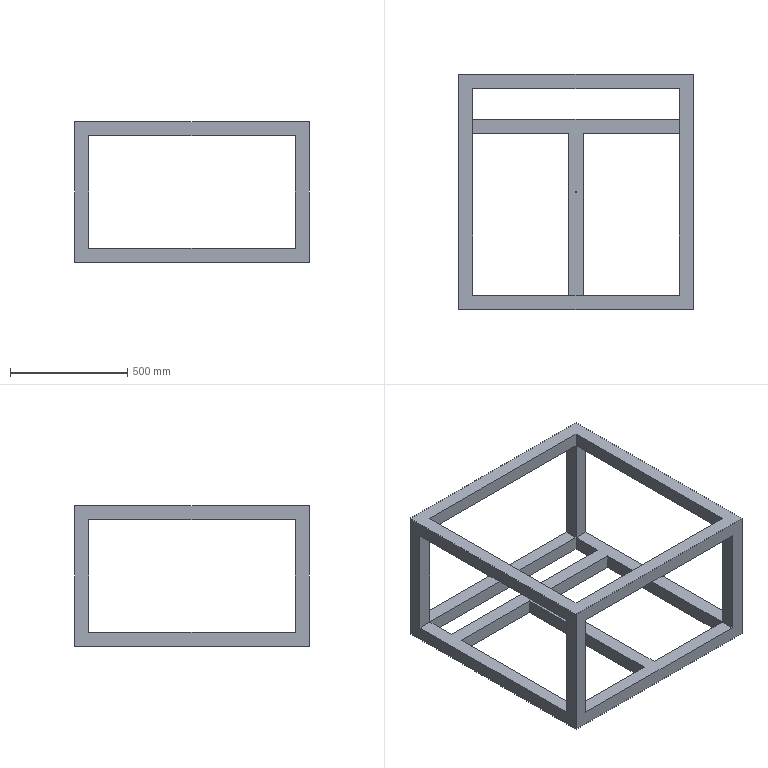Part | STEP file | Lower frame | 1 solid | 38 faces | box 1000 x 1000 x 600 mm | volume 39635953 mm3 | plane 36 | cylinder 2 | commonest cylinder face diameters 1 x2